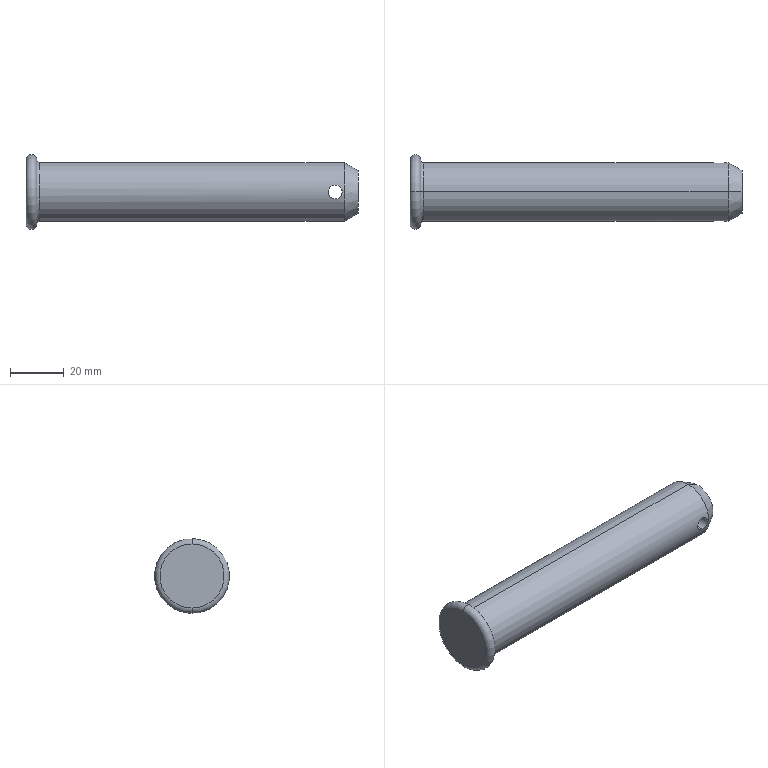Part | SolidWorks | features Chamfer 1, Cut 1, Fillet 1, Revolution 1 | 1 solid | 12 faces | box 124 x 28 x 28 mm | volume 46998 mm3 | cylinder 4 | torus 4 | cone 2 | plane 2 | commonest cylinder face diameters 5.18 x2 22 x2
STEP:
#1=CARTESIAN_POINT('',(115.5,-10.691,-2.59));
#2=VERTEX_POINT('',#1);
#3=CARTESIAN_POINT('',(115.5,-10.691,2.59));
#4=VERTEX_POINT('',#3);
#5=CARTESIAN_POINT('',(115.5,-10.691,-2.59));
#6=CARTESIAN_POINT('',(115.161,-10.691,-2.59));
#7=CARTESIAN_POINT('',(114.819,-10.708,-2.522));
#8=CARTESIAN_POINT('',(114.352,-10.751,-2.328));
#9=CARTESIAN_POINT('',(114.2,-10.769,-2.247));
#10=CARTESIAN_POINT('',(113.919,-10.806,-2.058));
#11=CARTESIAN_POINT('',(113.789,-10.826,-1.952));
#12=CARTESIAN_POINT('',(113.55,-10.866,-1.713));
#13=CARTESIAN_POINT('',(113.441,-10.887,-1.58));
#14=CARTESIAN_POINT('',(113.254,-10.924,-1.3));
#15=CARTESIAN_POINT('',(113.174,-10.941,-1.152));
#16=CARTESIAN_POINT('',(112.978,-10.984,-0.6798));
#17=CARTESIAN_POINT('',(112.91,-11.,-0.3427));
#18=CARTESIAN_POINT('',(112.91,-11.,0.1699));
#19=CARTESIAN_POINT('',(112.927,-10.996,0.3384));
#20=CARTESIAN_POINT('',(112.993,-10.981,0.6709));
#21=CARTESIAN_POINT('',(113.043,-10.969,0.8362));
#22=CARTESIAN_POINT('',(113.173,-10.941,1.149));
#23=CARTESIAN_POINT('',(113.252,-10.924,1.297));
#24=CARTESIAN_POINT('',(113.441,-10.887,1.58));
#25=CARTESIAN_POINT('',(113.549,-10.867,1.711));
#26=CARTESIAN_POINT('',(113.905,-10.806,2.068));
#27=CARTESIAN_POINT('',(114.193,-10.766,2.261));
#28=CARTESIAN_POINT('',(114.66,-10.723,2.456));
#29=CARTESIAN_POINT('',(114.825,-10.711,2.506));
#30=CARTESIAN_POINT('',(115.159,-10.695,2.573));
#31=CARTESIAN_POINT('',(115.328,-10.691,2.59));
#32=CARTESIAN_POINT('',(115.5,-10.691,2.59));
#33=B_SPLINE_CURVE_WITH_KNOTS('',3,(#5,#6,#7,#8,#9,#10,#11,#12,#13,#14,#15,#16,#17,#18,#19,#20,#21,#22,#23,#24,#25,#26,#27,#28,#29,#30,#31,#32),.UNSPECIFIED.,.F.,.F.,(4,2,2,2,2,2,2,2,2,2,2,2,2,4),(0.008126,0.009142,0.009649,0.01016,0.01066,0.01117,0.01219,0.0127,0.0132,0.01371,0.01422,0.01523,0.01574,0.01625),.UNSPECIFIED.);
#34=EDGE_CURVE('',#2,#4,#33,.T.);
#35=ORIENTED_EDGE('',*,*,#34,.F.);
#36=CARTESIAN_POINT('',(115.5,10.691,-2.59));
#37=VERTEX_POINT('',#36);
#38=CARTESIAN_POINT('',(115.5,-500.,-2.59));
#39=DIRECTION('',(0.,1.,0.));
#40=VECTOR('',#39,1000.);
#41=LINE('',#38,#40);
#42=EDGE_CURVE('',#2,#37,#41,.T.);
#43=ORIENTED_EDGE('',*,*,#42,.T.);
#44=CARTESIAN_POINT('',(115.5,10.691,2.59));
#45=VERTEX_POINT('',#44);
#46=CARTESIAN_POINT('',(115.5,10.691,2.59));
#47=CARTESIAN_POINT('',(115.328,10.691,2.59));
#48=CARTESIAN_POINT('',(115.159,10.695,2.573));
#49=CARTESIAN_POINT('',(114.828,10.711,2.507));
#50=CARTESIAN_POINT('',(114.663,10.722,2.457));
#51=CARTESIAN_POINT('',(114.349,10.751,2.327));
#52=CARTESIAN_POINT('',(114.201,10.768,2.247));
#53=CARTESIAN_POINT('',(113.92,10.806,2.059));
#54=CARTESIAN_POINT('',(113.787,10.826,1.95));
#55=CARTESIAN_POINT('',(113.43,10.887,1.593));
#56=CARTESIAN_POINT('',(113.237,10.927,1.305));
#57=CARTESIAN_POINT('',(113.043,10.969,0.8377));
#58=CARTESIAN_POINT('',(112.993,10.981,0.6738));
#59=CARTESIAN_POINT('',(112.927,10.996,0.3391));
#60=CARTESIAN_POINT('',(112.91,11.,0.1707));
#61=CARTESIAN_POINT('',(112.91,11.,-0.1686));
#62=CARTESIAN_POINT('',(112.927,10.996,-0.3409));
#63=CARTESIAN_POINT('',(112.993,10.981,-0.6736));
#64=CARTESIAN_POINT('',(113.043,10.969,-0.8353));
#65=CARTESIAN_POINT('',(113.238,10.927,-1.307));
#66=CARTESIAN_POINT('',(113.429,10.887,-1.592));
#67=CARTESIAN_POINT('',(113.789,10.826,-1.952));
#68=CARTESIAN_POINT('',(113.919,10.806,-2.059));
#69=CARTESIAN_POINT('',(114.199,10.769,-2.246));
#70=CARTESIAN_POINT('',(114.351,10.751,-2.327));
#71=CARTESIAN_POINT('',(114.664,10.722,-2.457));
#72=CARTESIAN_POINT('',(114.825,10.711,-2.506));
#73=CARTESIAN_POINT('',(115.159,10.695,-2.573));
#74=CARTESIAN_POINT('',(115.331,10.691,-2.59));
#75=CARTESIAN_POINT('',(115.5,10.691,-2.59));
#76=B_SPLINE_CURVE_WITH_KNOTS('',3,(#46,#47,#48,#49,#50,#51,#52,#53,#54,#55,#56,#57,#58,#59,#60,#61,#62,#63,#64,#65,#66,#67,#68,#69,#70,#71,#72,#73,#74,#75),.UNSPECIFIED.,.F.,.F.,(4,2,2,2,2,2,2,2,2,2,2,2,2,2,4),(0.,0.0005079,0.001016,0.001524,0.002032,0.003047,0.003555,0.004063,0.004571,0.005079,0.006095,0.006602,0.00711,0.007618,0.008126),.UNSPECIFIED.);
#77=EDGE_CURVE('',#45,#37,#76,.T.);
#78=ORIENTED_EDGE('',*,*,#77,.F.);
#79=CARTESIAN_POINT('',(115.5,-500.,2.59));
#80=DIRECTION('',(0.,1.,0.));
#81=VECTOR('',#80,1000.);
#82=LINE('',#79,#81);
#83=EDGE_CURVE('',#4,#45,#82,.T.);
#84=ORIENTED_EDGE('',*,*,#83,.F.);
#85=EDGE_LOOP('',(#35,#43,#78,#84));
#86=FACE_OUTER_BOUND('',#85,.T.);
#87=CARTESIAN_POINT('',(115.5,-500.,0.));
#88=DIRECTION('',(0.,1.,0.));
#89=DIRECTION('',(0.,0.,1.));
#90=AXIS2_PLACEMENT_3D('',#87,#88,#89);
#91=CYLINDRICAL_SURFACE('',#90,2.59);
#92=ADVANCED_FACE('',(#86),#91,.F.);
#93=CARTESIAN_POINT('',(124.,0.,-8.));
#94=VERTEX_POINT('',#93);
#95=CARTESIAN_POINT('',(124.,0.,8.));
#96=VERTEX_POINT('',#95);
#97=CARTESIAN_POINT('',(124.,0.,0.));
#98=DIRECTION('',(1.,0.,0.));
#99=DIRECTION('',(0.,0.,1.));
#100=AXIS2_PLACEMENT_3D('',#97,#98,#99);
#101=CIRCLE('',#100,8.);
#102=EDGE_CURVE('',#94,#96,#101,.T.);
#103=ORIENTED_EDGE('',*,*,#102,.F.);
#104=CARTESIAN_POINT('',(118.804,0.,-11.));
#105=VERTEX_POINT('',#104);
#106=CARTESIAN_POINT('',(118.804,0.,-11.));
#107=DIRECTION('',(-0.866,0.,-0.5));
#108=VECTOR('',#107,1000.);
#109=LINE('',#106,#108);
#110=EDGE_CURVE('',#94,#105,#109,.T.);
#111=ORIENTED_EDGE('',*,*,#110,.T.);
#112=CARTESIAN_POINT('',(118.804,0.,11.));
#113=VERTEX_POINT('',#112);
#114=CARTESIAN_POINT('',(118.804,0.,0.));
#115=DIRECTION('',(-1.,0.,0.));
#116=DIRECTION('',(0.,0.,1.));
#117=AXIS2_PLACEMENT_3D('',#114,#115,#116);
#118=CIRCLE('',#117,11.);
#119=EDGE_CURVE('',#113,#105,#118,.T.);
#120=ORIENTED_EDGE('',*,*,#119,.F.);
#121=CARTESIAN_POINT('',(118.804,0.,11.));
#122=DIRECTION('',(-0.866,0.,0.5));
#123=VECTOR('',#122,1000.);
#124=LINE('',#121,#123);
#125=EDGE_CURVE('',#96,#113,#124,.T.);
#126=ORIENTED_EDGE('',*,*,#125,.F.);
#127=EDGE_LOOP('',(#103,#111,#120,#126));
#128=FACE_OUTER_BOUND('',#127,.T.);
#129=CARTESIAN_POINT('',(118.804,0.,0.));
#130=DIRECTION('',(-1.,0.,0.));
#131=DIRECTION('',(0.,0.,1.));
#132=AXIS2_PLACEMENT_3D('',#129,#130,#131);
#133=CONICAL_SURFACE('',#132,11.,0.5236);
#134=ADVANCED_FACE('',(#128),#133,.T.);
#135=CARTESIAN_POINT('',(4.,0.,-12.));
#136=VERTEX_POINT('',#135);
#137=CARTESIAN_POINT('',(4.,0.,12.));
#138=VERTEX_POINT('',#137);
#139=CARTESIAN_POINT('',(4.,0.,0.));
#140=DIRECTION('',(-1.,0.,0.));
#141=DIRECTION('',(0.,0.,1.));
#142=AXIS2_PLACEMENT_3D('',#139,#140,#141);
#143=CIRCLE('',#142,12.);
#144=EDGE_CURVE('',#136,#138,#143,.T.);
#145=ORIENTED_EDGE('',*,*,#144,.F.);
#146=CARTESIAN_POINT('',(5.,0.,-11.));
#147=VERTEX_POINT('',#146);
#148=CARTESIAN_POINT('',(5.,0.,-12.));
#149=DIRECTION('',(0.,1.,0.));
#150=DIRECTION('',(0.,0.,1.));
#151=AXIS2_PLACEMENT_3D('',#148,#149,#150);
#152=CIRCLE('',#151,1.);
#153=EDGE_CURVE('',#136,#147,#152,.T.);
#154=ORIENTED_EDGE('',*,*,#153,.T.);
#155=CARTESIAN_POINT('',(5.,0.,11.));
#156=VERTEX_POINT('',#155);
#157=CARTESIAN_POINT('',(5.,0.,0.));
#158=DIRECTION('',(1.,0.,0.));
#159=DIRECTION('',(0.,0.,1.));
#160=AXIS2_PLACEMENT_3D('',#157,#158,#159);
#161=CIRCLE('',#160,11.);
#162=EDGE_CURVE('',#156,#147,#161,.T.);
#163=ORIENTED_EDGE('',*,*,#162,.F.);
#164=CARTESIAN_POINT('',(5.,0.,12.));
#165=DIRECTION('',(0.,-1.,0.));
#166=DIRECTION('',(0.,0.,-1.));
#167=AXIS2_PLACEMENT_3D('',#164,#165,#166);
#168=CIRCLE('',#167,1.);
#169=EDGE_CURVE('',#138,#156,#168,.T.);
#170=ORIENTED_EDGE('',*,*,#169,.F.);
#171=EDGE_LOOP('',(#145,#154,#163,#170));
#172=FACE_OUTER_BOUND('',#171,.T.);
#173=CARTESIAN_POINT('',(5.,0.,0.));
#174=DIRECTION('',(-1.,0.,0.));
#175=DIRECTION('',(0.,0.,1.));
#176=AXIS2_PLACEMENT_3D('',#173,#174,#175);
#177=TOROIDAL_SURFACE('',#176,12.,1.);
#178=ADVANCED_FACE('',(#172),#177,.F.);
#179=ORIENTED_EDGE('',*,*,#77,.T.);
#180=CARTESIAN_POINT('',(115.5,10.691,-2.59));
#181=CARTESIAN_POINT('',(115.839,10.691,-2.59));
#182=CARTESIAN_POINT('',(116.181,10.708,-2.522));
#183=CARTESIAN_POINT('',(116.648,10.751,-2.328));
#184=CARTESIAN_POINT('',(116.8,10.769,-2.247));
#185=CARTESIAN_POINT('',(117.081,10.806,-2.058));
#186=CARTESIAN_POINT('',(117.211,10.826,-1.952));
#187=CARTESIAN_POINT('',(117.45,10.866,-1.713));
#188=CARTESIAN_POINT('',(117.559,10.887,-1.58));
#189=CARTESIAN_POINT('',(117.746,10.924,-1.3));
#190=CARTESIAN_POINT('',(117.826,10.941,-1.152));
#191=CARTESIAN_POINT('',(118.022,10.984,-0.6798));
#192=CARTESIAN_POINT('',(118.09,11.,-0.3427));
#193=CARTESIAN_POINT('',(118.09,11.,0.1699));
#194=CARTESIAN_POINT('',(118.073,10.996,0.3384));
#195=CARTESIAN_POINT('',(118.007,10.981,0.6709));
#196=CARTESIAN_POINT('',(117.957,10.969,0.8362));
#197=CARTESIAN_POINT('',(117.827,10.941,1.149));
#198=CARTESIAN_POINT('',(117.748,10.924,1.297));
#199=CARTESIAN_POINT('',(117.559,10.887,1.58));
#200=CARTESIAN_POINT('',(117.451,10.867,1.711));
#201=CARTESIAN_POINT('',(117.095,10.806,2.068));
#202=CARTESIAN_POINT('',(116.807,10.766,2.261));
#203=CARTESIAN_POINT('',(116.34,10.723,2.456));
#204=CARTESIAN_POINT('',(116.175,10.711,2.506));
#205=CARTESIAN_POINT('',(115.841,10.695,2.573));
#206=CARTESIAN_POINT('',(115.672,10.691,2.59));
#207=CARTESIAN_POINT('',(115.5,10.691,2.59));
#208=B_SPLINE_CURVE_WITH_KNOTS('',3,(#180,#181,#182,#183,#184,#185,#186,#187,#188,#189,#190,#191,#192,#193,#194,#195,#196,#197,#198,#199,#200,#201,#202,#203,#204,#205,#206,#207),.UNSPECIFIED.,.F.,.F.,(4,2,2,2,2,2,2,2,2,2,2,2,2,4),(0.008126,0.009142,0.009649,0.01016,0.01066,0.01117,0.01219,0.0127,0.0132,0.01371,0.01422,0.01523,0.01574,0.01625),.UNSPECIFIED.);
#209=EDGE_CURVE('',#37,#45,#208,.T.);
#210=ORIENTED_EDGE('',*,*,#209,.T.);
#211=EDGE_LOOP('',(#179,#210));
#212=FACE_BOUND('',#211,.T.);
#213=ORIENTED_EDGE('',*,*,#119,.T.);
#214=CARTESIAN_POINT('',(0.,0.,-11.));
#215=DIRECTION('',(-1.,0.,0.));
#216=VECTOR('',#215,1000.);
#217=LINE('',#214,#216);
#218=EDGE_CURVE('',#105,#147,#217,.T.);
#219=ORIENTED_EDGE('',*,*,#218,.T.);
#220=CARTESIAN_POINT('',(5.,0.,0.));
#221=DIRECTION('',(1.,0.,0.));
#222=DIRECTION('',(0.,0.,1.));
#223=AXIS2_PLACEMENT_3D('',#220,#221,#222);
#224=CIRCLE('',#223,11.);
#225=EDGE_CURVE('',#147,#156,#224,.T.);
#226=ORIENTED_EDGE('',*,*,#225,.T.);
#227=CARTESIAN_POINT('',(0.,0.,11.));
#228=DIRECTION('',(-1.,0.,0.));
#229=VECTOR('',#228,1000.);
#230=LINE('',#227,#229);
#231=EDGE_CURVE('',#113,#156,#230,.T.);
#232=ORIENTED_EDGE('',*,*,#231,.F.);
#233=EDGE_LOOP('',(#213,#219,#226,#232));
#234=FACE_OUTER_BOUND('',#233,.T.);
#235=CARTESIAN_POINT('',(0.,0.,0.));
#236=DIRECTION('',(-1.,0.,0.));
#237=DIRECTION('',(0.,0.,1.));
#238=AXIS2_PLACEMENT_3D('',#235,#236,#237);
#239=CYLINDRICAL_SURFACE('',#238,11.);
#240=ADVANCED_FACE('',(#212,#234),#239,.T.);
#241=CARTESIAN_POINT('',(4.,0.,0.));
#242=DIRECTION('',(-1.,0.,0.));
#243=DIRECTION('',(0.,0.,1.));
#244=AXIS2_PLACEMENT_3D('',#241,#242,#243);
#245=CIRCLE('',#244,12.);
#246=EDGE_CURVE('',#138,#136,#245,.T.);
#247=ORIENTED_EDGE('',*,*,#246,.T.);
#248=CARTESIAN_POINT('',(0.,0.,-12.));
#249=VERTEX_POINT('',#248);
#250=CARTESIAN_POINT('',(2.,0.,-12.));
#251=DIRECTION('',(0.,1.,0.));
#252=DIRECTION('',(0.,0.,1.));
#253=AXIS2_PLACEMENT_3D('',#250,#251,#252);
#254=CIRCLE('',#253,2.);
#255=EDGE_CURVE('',#136,#249,#254,.T.);
#256=ORIENTED_EDGE('',*,*,#255,.T.);
#257=CARTESIAN_POINT('',(0.,0.,12.));
#258=VERTEX_POINT('',#257);
#259=CARTESIAN_POINT('',(0.,0.,0.));
#260=DIRECTION('',(-1.,0.,0.));
#261=DIRECTION('',(0.,0.,1.));
#262=AXIS2_PLACEMENT_3D('',#259,#260,#261);
#263=CIRCLE('',#262,12.);
#264=EDGE_CURVE('',#258,#249,#263,.T.);
#265=ORIENTED_EDGE('',*,*,#264,.F.);
#266=CARTESIAN_POINT('',(2.,0.,12.));
#267=DIRECTION('',(0.,-1.,0.));
#268=DIRECTION('',(0.,0.,-1.));
#269=AXIS2_PLACEMENT_3D('',#266,#267,#268);
#270=CIRCLE('',#269,2.);
#271=EDGE_CURVE('',#138,#258,#270,.T.);
#272=ORIENTED_EDGE('',*,*,#271,.F.);
#273=EDGE_LOOP('',(#247,#256,#265,#272));
#274=FACE_OUTER_BOUND('',#273,.T.);
#275=CARTESIAN_POINT('',(2.,0.,0.));
#276=DIRECTION('',(-1.,0.,0.));
#277=DIRECTION('',(0.,0.,1.));
#278=AXIS2_PLACEMENT_3D('',#275,#276,#277);
#279=TOROIDAL_SURFACE('',#278,12.,2.);
#280=ADVANCED_FACE('',(#274),#279,.T.);
#281=ORIENTED_EDGE('',*,*,#264,.T.);
#282=CARTESIAN_POINT('',(0.,0.,0.));
#283=DIRECTION('',(-1.,0.,0.));
#284=DIRECTION('',(0.,0.,1.));
#285=AXIS2_PLACEMENT_3D('',#282,#283,#284);
#286=CIRCLE('',#285,12.);
#287=EDGE_CURVE('',#249,#258,#286,.T.);
#288=ORIENTED_EDGE('',*,*,#287,.T.);
#289=EDGE_LOOP('',(#281,#288));
#290=FACE_OUTER_BOUND('',#289,.T.);
#291=CARTESIAN_POINT('',(0.,0.,0.));
#292=DIRECTION('',(1.,0.,0.));
#293=DIRECTION('',(0.,0.,-1.));
#294=AXIS2_PLACEMENT_3D('',#291,#292,#293);
#295=PLANE('',#294);
#296=ADVANCED_FACE('',(#290),#295,.F.);
#297=ORIENTED_EDGE('',*,*,#255,.F.);
#298=ORIENTED_EDGE('',*,*,#144,.T.);
#299=ORIENTED_EDGE('',*,*,#271,.T.);
#300=ORIENTED_EDGE('',*,*,#287,.F.);
#301=EDGE_LOOP('',(#297,#298,#299,#300));
#302=FACE_OUTER_BOUND('',#301,.T.);
#303=CARTESIAN_POINT('',(2.,0.,0.));
#304=DIRECTION('',(-1.,0.,0.));
#305=DIRECTION('',(0.,0.,1.));
#306=AXIS2_PLACEMENT_3D('',#303,#304,#305);
#307=TOROIDAL_SURFACE('',#306,12.,2.);
#308=ADVANCED_FACE('',(#302),#307,.T.);
#309=ORIENTED_EDGE('',*,*,#218,.F.);
#310=CARTESIAN_POINT('',(118.804,0.,0.));
#311=DIRECTION('',(-1.,0.,0.));
#312=DIRECTION('',(0.,0.,1.));
#313=AXIS2_PLACEMENT_3D('',#310,#311,#312);
#314=CIRCLE('',#313,11.);
#315=EDGE_CURVE('',#105,#113,#314,.T.);
#316=ORIENTED_EDGE('',*,*,#315,.T.);
#317=ORIENTED_EDGE('',*,*,#231,.T.);
#318=ORIENTED_EDGE('',*,*,#162,.T.);
#319=EDGE_LOOP('',(#309,#316,#317,#318));
#320=FACE_OUTER_BOUND('',#319,.T.);
#321=CARTESIAN_POINT('',(115.5,-10.691,2.59));
#322=CARTESIAN_POINT('',(115.672,-10.691,2.59));
#323=CARTESIAN_POINT('',(115.841,-10.695,2.573));
#324=CARTESIAN_POINT('',(116.172,-10.711,2.507));
#325=CARTESIAN_POINT('',(116.337,-10.722,2.457));
#326=CARTESIAN_POINT('',(116.651,-10.751,2.327));
#327=CARTESIAN_POINT('',(116.799,-10.768,2.247));
#328=CARTESIAN_POINT('',(117.08,-10.806,2.059));
#329=CARTESIAN_POINT('',(117.213,-10.826,1.95));
#330=CARTESIAN_POINT('',(117.57,-10.887,1.593));
#331=CARTESIAN_POINT('',(117.763,-10.927,1.305));
#332=CARTESIAN_POINT('',(117.957,-10.969,0.8377));
#333=CARTESIAN_POINT('',(118.007,-10.981,0.6738));
#334=CARTESIAN_POINT('',(118.073,-10.996,0.3391));
#335=CARTESIAN_POINT('',(118.09,-11.,0.1707));
#336=CARTESIAN_POINT('',(118.09,-11.,-0.1686));
#337=CARTESIAN_POINT('',(118.073,-10.996,-0.3409));
#338=CARTESIAN_POINT('',(118.007,-10.981,-0.6736));
#339=CARTESIAN_POINT('',(117.957,-10.969,-0.8353));
#340=CARTESIAN_POINT('',(117.762,-10.927,-1.307));
#341=CARTESIAN_POINT('',(117.571,-10.887,-1.592));
#342=CARTESIAN_POINT('',(117.211,-10.826,-1.952));
#343=CARTESIAN_POINT('',(117.081,-10.806,-2.059));
#344=CARTESIAN_POINT('',(116.801,-10.769,-2.246));
#345=CARTESIAN_POINT('',(116.649,-10.751,-2.327));
#346=CARTESIAN_POINT('',(116.336,-10.722,-2.457));
#347=CARTESIAN_POINT('',(116.175,-10.711,-2.506));
#348=CARTESIAN_POINT('',(115.841,-10.695,-2.573));
#349=CARTESIAN_POINT('',(115.669,-10.691,-2.59));
#350=CARTESIAN_POINT('',(115.5,-10.691,-2.59));
#351=B_SPLINE_CURVE_WITH_KNOTS('',3,(#321,#322,#323,#324,#325,#326,#327,#328,#329,#330,#331,#332,#333,#334,#335,#336,#337,#338,#339,#340,#341,#342,#343,#344,#345,#346,#347,#348,#349,#350),.UNSPECIFIED.,.F.,.F.,(4,2,2,2,2,2,2,2,2,2,2,2,2,2,4),(0.,0.0005079,0.001016,0.001524,0.002032,0.003047,0.003555,0.004063,0.004571,0.005079,0.006095,0.006602,0.00711,0.007618,0.008126),.UNSPECIFIED.);
#352=EDGE_CURVE('',#4,#2,#351,.T.);
#353=ORIENTED_EDGE('',*,*,#352,.T.);
#354=ORIENTED_EDGE('',*,*,#34,.T.);
#355=EDGE_LOOP('',(#353,#354));
#356=FACE_BOUND('',#355,.T.);
#357=CARTESIAN_POINT('',(0.,0.,0.));
#358=DIRECTION('',(-1.,0.,0.));
#359=DIRECTION('',(0.,0.,1.));
#360=AXIS2_PLACEMENT_3D('',#357,#358,#359);
#361=CYLINDRICAL_SURFACE('',#360,11.);
#362=ADVANCED_FACE('',(#320,#356),#361,.T.);
#363=CARTESIAN_POINT('',(124.,0.,0.));
#364=DIRECTION('',(1.,0.,0.));
#365=DIRECTION('',(0.,0.,1.));
#366=AXIS2_PLACEMENT_3D('',#363,#364,#365);
#367=CIRCLE('',#366,8.);
#368=EDGE_CURVE('',#96,#94,#367,.T.);
#369=ORIENTED_EDGE('',*,*,#368,.T.);
#370=ORIENTED_EDGE('',*,*,#102,.T.);
#371=EDGE_LOOP('',(#369,#370));
#372=FACE_OUTER_BOUND('',#371,.T.);
#373=CARTESIAN_POINT('',(124.,11.,0.));
#374=DIRECTION('',(-1.,0.,0.));
#375=DIRECTION('',(0.,0.,1.));
#376=AXIS2_PLACEMENT_3D('',#373,#374,#375);
#377=PLANE('',#376);
#378=ADVANCED_FACE('',(#372),#377,.F.);
#379=ORIENTED_EDGE('',*,*,#153,.F.);
#380=ORIENTED_EDGE('',*,*,#246,.F.);
#381=ORIENTED_EDGE('',*,*,#169,.T.);
#382=ORIENTED_EDGE('',*,*,#225,.F.);
#383=EDGE_LOOP('',(#379,#380,#381,#382));
#384=FACE_OUTER_BOUND('',#383,.T.);
#385=CARTESIAN_POINT('',(5.,0.,0.));
#386=DIRECTION('',(-1.,0.,0.));
#387=DIRECTION('',(0.,0.,1.));
#388=AXIS2_PLACEMENT_3D('',#385,#386,#387);
#389=TOROIDAL_SURFACE('',#388,12.,1.);
#390=ADVANCED_FACE('',(#384),#389,.F.);
#391=ORIENTED_EDGE('',*,*,#110,.F.);
#392=ORIENTED_EDGE('',*,*,#368,.F.);
#393=ORIENTED_EDGE('',*,*,#125,.T.);
#394=ORIENTED_EDGE('',*,*,#315,.F.);
#395=EDGE_LOOP('',(#391,#392,#393,#394));
#396=FACE_OUTER_BOUND('',#395,.T.);
#397=CARTESIAN_POINT('',(118.804,0.,0.));
#398=DIRECTION('',(-1.,0.,0.));
#399=DIRECTION('',(0.,0.,1.));
#400=AXIS2_PLACEMENT_3D('',#397,#398,#399);
#401=CONICAL_SURFACE('',#400,11.,0.5236);
#402=ADVANCED_FACE('',(#396),#401,.T.);
#403=ORIENTED_EDGE('',*,*,#42,.F.);
#404=ORIENTED_EDGE('',*,*,#352,.F.);
#405=ORIENTED_EDGE('',*,*,#83,.T.);
#406=ORIENTED_EDGE('',*,*,#209,.F.);
#407=EDGE_LOOP('',(#403,#404,#405,#406));
#408=FACE_OUTER_BOUND('',#407,.T.);
#409=CARTESIAN_POINT('',(115.5,-500.,0.));
#410=DIRECTION('',(0.,1.,0.));
#411=DIRECTION('',(0.,0.,1.));
#412=AXIS2_PLACEMENT_3D('',#409,#410,#411);
#413=CYLINDRICAL_SURFACE('',#412,2.59);
#414=ADVANCED_FACE('',(#408),#413,.F.);
#415=CLOSED_SHELL('',(#92,#134,#178,#240,#280,#296,#308,#362,#378,#390,#402,#414));
#416=MANIFOLD_SOLID_BREP('',#415);
#417=CARTESIAN_POINT('',(0.,0.,0.));
#418=DIRECTION('',(0.,0.,1.));
#419=DIRECTION('',(1.,0.,0.));
#420=AXIS2_PLACEMENT_3D('',#417,#418,#419);
#421=(LENGTH_UNIT()NAMED_UNIT(*)SI_UNIT(.MILLI.,.METRE.));
#422=UNCERTAINTY_MEASURE_WITH_UNIT(LENGTH_MEASURE(0.00001),#421,'','');
#423=(NAMED_UNIT(*)PLANE_ANGLE_UNIT()SI_UNIT($,.RADIAN.));
#424=(NAMED_UNIT(*)SI_UNIT($,.STERADIAN.)SOLID_ANGLE_UNIT());
#425=(GEOMETRIC_REPRESENTATION_CONTEXT(3)GLOBAL_UNCERTAINTY_ASSIGNED_CONTEXT((#422))GLOBAL_UNIT_ASSIGNED_CONTEXT((#421,#423,#424))REPRESENTATION_CONTEXT('',''));
#426=ADVANCED_BREP_SHAPE_REPRESENTATION('',(#416,#420),#425);